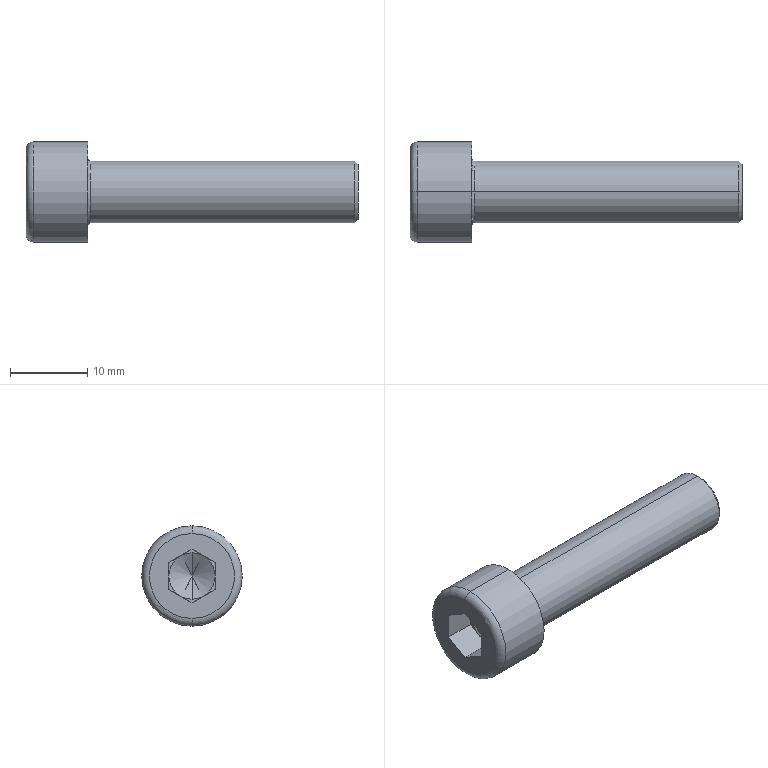Part | SolidWorks | features BaseBody 1 | 1 solid | 27 faces | box 43 x 13 x 13 mm | volume 2671 mm3 | plane 15 | cylinder 4 | torus 4 | cone 4 | commonest cylinder face diameters 8 x2 13 x2
STEP:
#1=CARTESIAN_POINT('',(42.6,0.,4.));
#2=VERTEX_POINT('',#1);
#3=CARTESIAN_POINT('',(42.6,0.,-4.));
#4=VERTEX_POINT('',#3);
#5=CARTESIAN_POINT('',(42.6,0.,0.));
#6=DIRECTION('',(-1.,0.,0.));
#7=DIRECTION('',(0.,0.,1.));
#8=AXIS2_PLACEMENT_3D('',#5,#6,#7);
#9=CIRCLE('',#8,4.);
#10=EDGE_CURVE('',#2,#4,#9,.T.);
#11=ORIENTED_EDGE('',*,*,#10,.T.);
#12=CARTESIAN_POINT('',(8.4,0.,-4.));
#13=VERTEX_POINT('',#12);
#14=CARTESIAN_POINT('',(43.,0.,-4.));
#15=DIRECTION('',(-1.,0.,0.));
#16=VECTOR('',#15,1000.);
#17=LINE('',#14,#16);
#18=EDGE_CURVE('',#4,#13,#17,.T.);
#19=ORIENTED_EDGE('',*,*,#18,.T.);
#20=CARTESIAN_POINT('',(8.4,0.,4.));
#21=VERTEX_POINT('',#20);
#22=CARTESIAN_POINT('',(8.4,0.,0.));
#23=DIRECTION('',(1.,0.,0.));
#24=DIRECTION('',(0.,0.,1.));
#25=AXIS2_PLACEMENT_3D('',#22,#23,#24);
#26=CIRCLE('',#25,4.);
#27=EDGE_CURVE('',#13,#21,#26,.T.);
#28=ORIENTED_EDGE('',*,*,#27,.T.);
#29=CARTESIAN_POINT('',(43.,0.,4.));
#30=DIRECTION('',(-1.,0.,0.));
#31=VECTOR('',#30,1000.);
#32=LINE('',#29,#31);
#33=EDGE_CURVE('',#2,#21,#32,.T.);
#34=ORIENTED_EDGE('',*,*,#33,.F.);
#35=EDGE_LOOP('',(#11,#19,#28,#34));
#36=FACE_OUTER_BOUND('',#35,.T.);
#37=CARTESIAN_POINT('',(43.,0.,0.));
#38=DIRECTION('',(-1.,0.,0.));
#39=DIRECTION('',(0.,0.,1.));
#40=AXIS2_PLACEMENT_3D('',#37,#38,#39);
#41=CYLINDRICAL_SURFACE('',#40,4.);
#42=ADVANCED_FACE('',(#36),#41,.T.);
#43=CARTESIAN_POINT('',(8.4,0.,0.));
#44=DIRECTION('',(1.,0.,0.));
#45=DIRECTION('',(0.,0.,1.));
#46=AXIS2_PLACEMENT_3D('',#43,#44,#45);
#47=CIRCLE('',#46,4.);
#48=EDGE_CURVE('',#21,#13,#47,.T.);
#49=ORIENTED_EDGE('',*,*,#48,.F.);
#50=CARTESIAN_POINT('',(8.,0.,4.4));
#51=VERTEX_POINT('',#50);
#52=CARTESIAN_POINT('',(8.4,0.,4.4));
#53=DIRECTION('',(0.,1.,0.));
#54=DIRECTION('',(0.,0.,1.));
#55=AXIS2_PLACEMENT_3D('',#52,#53,#54);
#56=CIRCLE('',#55,0.4);
#57=EDGE_CURVE('',#21,#51,#56,.T.);
#58=ORIENTED_EDGE('',*,*,#57,.T.);
#59=CARTESIAN_POINT('',(8.,0.,-4.4));
#60=VERTEX_POINT('',#59);
#61=CARTESIAN_POINT('',(8.,0.,-4.4));
#62=CARTESIAN_POINT('',(8.,-0.2798,-4.4));
#63=CARTESIAN_POINT('',(8.,-0.692,-4.361));
#64=CARTESIAN_POINT('',(8.,-1.16,-4.249));
#65=CARTESIAN_POINT('',(8.,-1.391,-4.175));
#66=CARTESIAN_POINT('',(8.,-1.489,-4.141));
#67=CARTESIAN_POINT('',(8.,-1.555,-4.116));
#68=CARTESIAN_POINT('',(8.,-1.585,-4.105));
#69=CARTESIAN_POINT('',(8.,-1.758,-4.036));
#70=CARTESIAN_POINT('',(8.,-1.96,-3.945));
#71=CARTESIAN_POINT('',(8.,-2.154,-3.837));
#72=CARTESIAN_POINT('',(8.,-2.282,-3.763));
#73=CARTESIAN_POINT('',(8.,-2.344,-3.724));
#74=CARTESIAN_POINT('',(8.,-2.661,-3.517));
#75=CARTESIAN_POINT('',(8.,-2.897,-3.326));
#76=CARTESIAN_POINT('',(8.,-3.218,-3.004));
#77=CARTESIAN_POINT('',(8.,-3.37,-2.836));
#78=CARTESIAN_POINT('',(8.,-3.509,-2.656));
#79=CARTESIAN_POINT('',(8.,-3.598,-2.534));
#80=CARTESIAN_POINT('',(8.,-3.642,-2.47));
#81=CARTESIAN_POINT('',(8.,-3.764,-2.284));
#82=CARTESIAN_POINT('',(8.,-3.876,-2.092));
#83=CARTESIAN_POINT('',(8.,-3.989,-1.859));
#84=CARTESIAN_POINT('',(8.,-4.042,-1.74));
#85=CARTESIAN_POINT('',(8.,-4.063,-1.689));
#86=CARTESIAN_POINT('',(8.,-4.077,-1.654));
#87=CARTESIAN_POINT('',(8.,-4.085,-1.636));
#88=CARTESIAN_POINT('',(8.,-4.297,-1.1));
#89=CARTESIAN_POINT('',(8.,-4.4,-0.5588));
#90=CARTESIAN_POINT('',(8.,-4.4,0.2794));
#91=CARTESIAN_POINT('',(8.,-4.361,0.6914));
#92=CARTESIAN_POINT('',(8.,-4.249,1.16));
#93=CARTESIAN_POINT('',(8.,-4.176,1.391));
#94=CARTESIAN_POINT('',(8.,-4.141,1.489));
#95=CARTESIAN_POINT('',(8.,-4.116,1.554));
#96=CARTESIAN_POINT('',(8.,-4.105,1.585));
#97=CARTESIAN_POINT('',(8.,-4.036,1.758));
#98=CARTESIAN_POINT('',(8.,-3.945,1.96));
#99=CARTESIAN_POINT('',(8.,-3.837,2.154));
#100=CARTESIAN_POINT('',(8.,-3.763,2.282));
#101=CARTESIAN_POINT('',(8.,-3.724,2.344));
#102=CARTESIAN_POINT('',(8.,-3.517,2.661));
#103=CARTESIAN_POINT('',(8.,-3.326,2.897));
#104=CARTESIAN_POINT('',(8.,-3.004,3.218));
#105=CARTESIAN_POINT('',(8.,-2.836,3.37));
#106=CARTESIAN_POINT('',(8.,-2.656,3.509));
#107=CARTESIAN_POINT('',(8.,-2.534,3.598));
#108=CARTESIAN_POINT('',(8.,-2.47,3.642));
#109=CARTESIAN_POINT('',(8.,-2.284,3.764));
#110=CARTESIAN_POINT('',(8.,-2.092,3.876));
#111=CARTESIAN_POINT('',(8.,-1.859,3.989));
#112=CARTESIAN_POINT('',(8.,-1.74,4.042));
#113=CARTESIAN_POINT('',(8.,-1.689,4.063));
#114=CARTESIAN_POINT('',(8.,-1.654,4.077));
#115=CARTESIAN_POINT('',(8.,-1.636,4.085));
#116=CARTESIAN_POINT('',(8.,-1.1,4.297));
#117=CARTESIAN_POINT('',(8.,-0.5602,4.4));
#118=CARTESIAN_POINT('',(8.,0.,4.4));
#119=B_SPLINE_CURVE_WITH_KNOTS('',3,(#61,#62,#63,#64,#65,#66,#67,#68,#69,#70,#71,#72,#73,#74,#75,#76,#77,#78,#79,#80,#81,#82,#83,#84,#85,#86,#87,#88,#89,#90,#91,#92,#93,#94,#95,#96,#97,#98,#99,#100,#101,#102,#103,#104,#105,#106,#107,#108,#109,#110,#111,#112,#113,#114,#115,#116,#117,#118),.UNSPECIFIED.,.F.,.F.,(4,1,1,1,2,2,1,2,2,2,1,2,2,1,1,1,2,2,2,1,1,1,2,2,1,2,2,2,1,2,2,1,1,1,2,2,4),(0.,0.0625,0.09375,0.1094,0.1172,0.125,0.1563,0.1719,0.1875,0.25,0.2813,0.2969,0.3125,0.3438,0.3594,0.3672,0.3711,0.375,0.5,0.5625,0.5937,0.6094,0.6172,0.625,0.6562,0.6719,0.6875,0.75,0.7813,0.7969,0.8125,0.8438,0.8594,0.8672,0.8711,0.875,1.),.UNSPECIFIED.);
#120=EDGE_CURVE('',#60,#51,#119,.T.);
#121=ORIENTED_EDGE('',*,*,#120,.F.);
#122=CARTESIAN_POINT('',(8.4,0.,-4.4));
#123=DIRECTION('',(0.,-1.,0.));
#124=DIRECTION('',(0.,0.,-1.));
#125=AXIS2_PLACEMENT_3D('',#122,#123,#124);
#126=CIRCLE('',#125,0.4);
#127=EDGE_CURVE('',#13,#60,#126,.T.);
#128=ORIENTED_EDGE('',*,*,#127,.F.);
#129=EDGE_LOOP('',(#49,#58,#121,#128));
#130=FACE_OUTER_BOUND('',#129,.T.);
#131=CARTESIAN_POINT('',(8.4,0.,0.));
#132=DIRECTION('',(1.,0.,0.));
#133=DIRECTION('',(0.,0.,-1.));
#134=AXIS2_PLACEMENT_3D('',#131,#132,#133);
#135=TOROIDAL_SURFACE('',#134,4.4,0.4);
#136=ADVANCED_FACE('',(#130),#135,.F.);
#137=CARTESIAN_POINT('',(43.,0.,3.6));
#138=VERTEX_POINT('',#137);
#139=CARTESIAN_POINT('',(43.,0.,-3.6));
#140=VERTEX_POINT('',#139);
#141=CARTESIAN_POINT('',(43.,0.,0.));
#142=DIRECTION('',(-1.,0.,0.));
#143=DIRECTION('',(0.,0.,1.));
#144=AXIS2_PLACEMENT_3D('',#141,#142,#143);
#145=CIRCLE('',#144,3.6);
#146=EDGE_CURVE('',#138,#140,#145,.T.);
#147=ORIENTED_EDGE('',*,*,#146,.T.);
#148=CARTESIAN_POINT('',(42.6,0.,-4.));
#149=DIRECTION('',(-0.7071,0.,-0.7071));
#150=VECTOR('',#149,1000.);
#151=LINE('',#148,#150);
#152=EDGE_CURVE('',#140,#4,#151,.T.);
#153=ORIENTED_EDGE('',*,*,#152,.T.);
#154=ORIENTED_EDGE('',*,*,#10,.F.);
#155=CARTESIAN_POINT('',(42.6,0.,4.));
#156=DIRECTION('',(-0.7071,0.,0.7071));
#157=VECTOR('',#156,1000.);
#158=LINE('',#155,#157);
#159=EDGE_CURVE('',#138,#2,#158,.T.);
#160=ORIENTED_EDGE('',*,*,#159,.F.);
#161=EDGE_LOOP('',(#147,#153,#154,#160));
#162=FACE_OUTER_BOUND('',#161,.T.);
#163=CARTESIAN_POINT('',(42.6,0.,0.));
#164=DIRECTION('',(-1.,0.,0.));
#165=DIRECTION('',(0.,0.,1.));
#166=AXIS2_PLACEMENT_3D('',#163,#164,#165);
#167=CONICAL_SURFACE('',#166,4.,0.7854);
#168=ADVANCED_FACE('',(#162),#167,.T.);
#169=CARTESIAN_POINT('',(8.,0.,-6.5));
#170=VERTEX_POINT('',#169);
#171=CARTESIAN_POINT('',(8.,0.,6.5));
#172=VERTEX_POINT('',#171);
#173=CARTESIAN_POINT('',(8.,0.,0.));
#174=DIRECTION('',(1.,0.,0.));
#175=DIRECTION('',(0.,0.,1.));
#176=AXIS2_PLACEMENT_3D('',#173,#174,#175);
#177=CIRCLE('',#176,6.5);
#178=EDGE_CURVE('',#170,#172,#177,.T.);
#179=ORIENTED_EDGE('',*,*,#178,.F.);
#180=CARTESIAN_POINT('',(1.,0.,-6.5));
#181=VERTEX_POINT('',#180);
#182=CARTESIAN_POINT('',(8.,0.,-6.5));
#183=DIRECTION('',(-1.,0.,0.));
#184=VECTOR('',#183,1000.);
#185=LINE('',#182,#184);
#186=EDGE_CURVE('',#170,#181,#185,.T.);
#187=ORIENTED_EDGE('',*,*,#186,.T.);
#188=CARTESIAN_POINT('',(1.,0.,6.5));
#189=VERTEX_POINT('',#188);
#190=CARTESIAN_POINT('',(1.,0.,0.));
#191=DIRECTION('',(1.,0.,0.));
#192=DIRECTION('',(0.,0.,1.));
#193=AXIS2_PLACEMENT_3D('',#190,#191,#192);
#194=CIRCLE('',#193,6.5);
#195=EDGE_CURVE('',#181,#189,#194,.T.);
#196=ORIENTED_EDGE('',*,*,#195,.T.);
#197=CARTESIAN_POINT('',(8.,0.,6.5));
#198=DIRECTION('',(-1.,0.,0.));
#199=VECTOR('',#198,1000.);
#200=LINE('',#197,#199);
#201=EDGE_CURVE('',#172,#189,#200,.T.);
#202=ORIENTED_EDGE('',*,*,#201,.F.);
#203=EDGE_LOOP('',(#179,#187,#196,#202));
#204=FACE_OUTER_BOUND('',#203,.T.);
#205=CARTESIAN_POINT('',(8.,0.,0.));
#206=DIRECTION('',(-1.,0.,0.));
#207=DIRECTION('',(0.,0.,1.));
#208=AXIS2_PLACEMENT_3D('',#205,#206,#207);
#209=CYLINDRICAL_SURFACE('',#208,6.5);
#210=ADVANCED_FACE('',(#204),#209,.T.);
#211=CARTESIAN_POINT('',(0.,0.,-5.5));
#212=VERTEX_POINT('',#211);
#213=CARTESIAN_POINT('',(0.,0.,5.5));
#214=VERTEX_POINT('',#213);
#215=CARTESIAN_POINT('',(0.,0.,0.));
#216=DIRECTION('',(1.,0.,0.));
#217=DIRECTION('',(0.,0.,-1.));
#218=AXIS2_PLACEMENT_3D('',#215,#216,#217);
#219=CIRCLE('',#218,5.5);
#220=EDGE_CURVE('',#212,#214,#219,.T.);
#221=ORIENTED_EDGE('',*,*,#220,.T.);
#222=CARTESIAN_POINT('',(1.,0.,5.5));
#223=DIRECTION('',(0.,1.,0.));
#224=DIRECTION('',(0.,0.,1.));
#225=AXIS2_PLACEMENT_3D('',#222,#223,#224);
#226=CIRCLE('',#225,1.);
#227=EDGE_CURVE('',#214,#189,#226,.T.);
#228=ORIENTED_EDGE('',*,*,#227,.T.);
#229=ORIENTED_EDGE('',*,*,#195,.F.);
#230=CARTESIAN_POINT('',(1.,0.,-5.5));
#231=DIRECTION('',(0.,-1.,0.));
#232=DIRECTION('',(0.,0.,-1.));
#233=AXIS2_PLACEMENT_3D('',#230,#231,#232);
#234=CIRCLE('',#233,1.);
#235=EDGE_CURVE('',#212,#181,#234,.T.);
#236=ORIENTED_EDGE('',*,*,#235,.F.);
#237=EDGE_LOOP('',(#221,#228,#229,#236));
#238=FACE_OUTER_BOUND('',#237,.T.);
#239=CARTESIAN_POINT('',(1.,0.,0.));
#240=DIRECTION('',(1.,0.,0.));
#241=DIRECTION('',(0.,0.,-1.));
#242=AXIS2_PLACEMENT_3D('',#239,#240,#241);
#243=TOROIDAL_SURFACE('',#242,5.5,1.);
#244=ADVANCED_FACE('',(#238),#243,.T.);
#245=CARTESIAN_POINT('',(5.732,0.,0.));
#246=VERTEX_POINT('',#245);
#247=CARTESIAN_POINT('',(4.,0.,3.));
#248=VERTEX_POINT('',#247);
#249=CARTESIAN_POINT('',(4.,0.,3.));
#250=DIRECTION('',(-0.5,0.,0.866));
#251=VECTOR('',#250,1000.);
#252=LINE('',#249,#251);
#253=EDGE_CURVE('',#246,#248,#252,.T.);
#254=ORIENTED_EDGE('',*,*,#253,.F.);
#255=CARTESIAN_POINT('',(4.,0.,-3.));
#256=VERTEX_POINT('',#255);
#257=CARTESIAN_POINT('',(4.,0.,-3.));
#258=DIRECTION('',(-0.5,0.,-0.866));
#259=VECTOR('',#258,1000.);
#260=LINE('',#257,#259);
#261=EDGE_CURVE('',#246,#256,#260,.T.);
#262=ORIENTED_EDGE('',*,*,#261,.T.);
#263=CARTESIAN_POINT('',(4.,-1.5,-2.598));
#264=VERTEX_POINT('',#263);
#265=CARTESIAN_POINT('',(4.,0.,0.));
#266=DIRECTION('',(1.,0.,0.));
#267=DIRECTION('',(0.,0.,1.));
#268=AXIS2_PLACEMENT_3D('',#265,#266,#267);
#269=CIRCLE('',#268,3.);
#270=EDGE_CURVE('',#264,#256,#269,.T.);
#271=ORIENTED_EDGE('',*,*,#270,.F.);
#272=CARTESIAN_POINT('',(4.,-3.,0.));
#273=VERTEX_POINT('',#272);
#274=CARTESIAN_POINT('',(4.,0.,0.));
#275=DIRECTION('',(-1.,0.,0.));
#276=DIRECTION('',(0.,0.,1.));
#277=AXIS2_PLACEMENT_3D('',#274,#275,#276);
#278=CIRCLE('',#277,3.);
#279=EDGE_CURVE('',#264,#273,#278,.T.);
#280=ORIENTED_EDGE('',*,*,#279,.T.);
#281=CARTESIAN_POINT('',(4.,-1.5,2.598));
#282=VERTEX_POINT('',#281);
#283=CARTESIAN_POINT('',(4.,0.,0.));
#284=DIRECTION('',(1.,0.,0.));
#285=DIRECTION('',(0.,0.,1.));
#286=AXIS2_PLACEMENT_3D('',#283,#284,#285);
#287=CIRCLE('',#286,3.);
#288=EDGE_CURVE('',#282,#273,#287,.T.);
#289=ORIENTED_EDGE('',*,*,#288,.F.);
#290=CARTESIAN_POINT('',(4.,0.,0.));
#291=DIRECTION('',(1.,0.,0.));
#292=DIRECTION('',(0.,0.,1.));
#293=AXIS2_PLACEMENT_3D('',#290,#291,#292);
#294=CIRCLE('',#293,3.);
#295=EDGE_CURVE('',#248,#282,#294,.T.);
#296=ORIENTED_EDGE('',*,*,#295,.F.);
#297=EDGE_LOOP('',(#254,#262,#271,#280,#289,#296));
#298=FACE_OUTER_BOUND('',#297,.T.);
#299=CARTESIAN_POINT('',(4.,0.,0.));
#300=DIRECTION('',(-1.,0.,0.));
#301=DIRECTION('',(0.,0.,1.));
#302=AXIS2_PLACEMENT_3D('',#299,#300,#301);
#303=CONICAL_SURFACE('',#302,3.,1.047);
#304=ADVANCED_FACE('',(#298),#303,.F.);
#305=ORIENTED_EDGE('',*,*,#18,.F.);
#306=CARTESIAN_POINT('',(42.6,0.,0.));
#307=DIRECTION('',(-1.,0.,0.));
#308=DIRECTION('',(0.,0.,1.));
#309=AXIS2_PLACEMENT_3D('',#306,#307,#308);
#310=CIRCLE('',#309,4.);
#311=EDGE_CURVE('',#4,#2,#310,.T.);
#312=ORIENTED_EDGE('',*,*,#311,.T.);
#313=ORIENTED_EDGE('',*,*,#33,.T.);
#314=ORIENTED_EDGE('',*,*,#48,.T.);
#315=EDGE_LOOP('',(#305,#312,#313,#314));
#316=FACE_OUTER_BOUND('',#315,.T.);
#317=CARTESIAN_POINT('',(43.,0.,0.));
#318=DIRECTION('',(-1.,0.,0.));
#319=DIRECTION('',(0.,0.,1.));
#320=AXIS2_PLACEMENT_3D('',#317,#318,#319);
#321=CYLINDRICAL_SURFACE('',#320,4.);
#322=ADVANCED_FACE('',(#316),#321,.T.);
#323=ORIENTED_EDGE('',*,*,#57,.F.);
#324=ORIENTED_EDGE('',*,*,#27,.F.);
#325=ORIENTED_EDGE('',*,*,#127,.T.);
#326=CARTESIAN_POINT('',(8.,0.,4.4));
#327=CARTESIAN_POINT('',(8.,0.2798,4.4));
#328=CARTESIAN_POINT('',(8.,0.692,4.361));
#329=CARTESIAN_POINT('',(8.,1.16,4.249));
#330=CARTESIAN_POINT('',(8.,1.391,4.175));
#331=CARTESIAN_POINT('',(8.,1.489,4.141));
#332=CARTESIAN_POINT('',(8.,1.555,4.116));
#333=CARTESIAN_POINT('',(8.,1.585,4.105));
#334=CARTESIAN_POINT('',(8.,1.758,4.036));
#335=CARTESIAN_POINT('',(8.,1.96,3.945));
#336=CARTESIAN_POINT('',(8.,2.154,3.837));
#337=CARTESIAN_POINT('',(8.,2.282,3.763));
#338=CARTESIAN_POINT('',(8.,2.344,3.724));
#339=CARTESIAN_POINT('',(8.,2.661,3.517));
#340=CARTESIAN_POINT('',(8.,2.897,3.326));
#341=CARTESIAN_POINT('',(8.,3.218,3.004));
#342=CARTESIAN_POINT('',(8.,3.37,2.836));
#343=CARTESIAN_POINT('',(8.,3.509,2.656));
#344=CARTESIAN_POINT('',(8.,3.598,2.534));
#345=CARTESIAN_POINT('',(8.,3.642,2.47));
#346=CARTESIAN_POINT('',(8.,3.764,2.284));
#347=CARTESIAN_POINT('',(8.,3.876,2.092));
#348=CARTESIAN_POINT('',(8.,3.989,1.859));
#349=CARTESIAN_POINT('',(8.,4.042,1.74));
#350=CARTESIAN_POINT('',(8.,4.063,1.689));
#351=CARTESIAN_POINT('',(8.,4.077,1.654));
#352=CARTESIAN_POINT('',(8.,4.085,1.636));
#353=CARTESIAN_POINT('',(8.,4.297,1.1));
#354=CARTESIAN_POINT('',(8.,4.4,0.5588));
#355=CARTESIAN_POINT('',(8.,4.4,-0.2794));
#356=CARTESIAN_POINT('',(8.,4.361,-0.6914));
#357=CARTESIAN_POINT('',(8.,4.249,-1.16));
#358=CARTESIAN_POINT('',(8.,4.176,-1.391));
#359=CARTESIAN_POINT('',(8.,4.141,-1.489));
#360=CARTESIAN_POINT('',(8.,4.116,-1.554));
#361=CARTESIAN_POINT('',(8.,4.105,-1.585));
#362=CARTESIAN_POINT('',(8.,4.036,-1.758));
#363=CARTESIAN_POINT('',(8.,3.945,-1.96));
#364=CARTESIAN_POINT('',(8.,3.837,-2.154));
#365=CARTESIAN_POINT('',(8.,3.763,-2.282));
#366=CARTESIAN_POINT('',(8.,3.724,-2.344));
#367=CARTESIAN_POINT('',(8.,3.517,-2.661));
#368=CARTESIAN_POINT('',(8.,3.326,-2.897));
#369=CARTESIAN_POINT('',(8.,3.004,-3.218));
#370=CARTESIAN_POINT('',(8.,2.836,-3.37));
#371=CARTESIAN_POINT('',(8.,2.656,-3.509));
#372=CARTESIAN_POINT('',(8.,2.534,-3.598));
#373=CARTESIAN_POINT('',(8.,2.47,-3.642));
#374=CARTESIAN_POINT('',(8.,2.284,-3.764));
#375=CARTESIAN_POINT('',(8.,2.092,-3.876));
#376=CARTESIAN_POINT('',(8.,1.859,-3.989));
#377=CARTESIAN_POINT('',(8.,1.74,-4.042));
#378=CARTESIAN_POINT('',(8.,1.689,-4.063));
#379=CARTESIAN_POINT('',(8.,1.654,-4.077));
#380=CARTESIAN_POINT('',(8.,1.636,-4.085));
#381=CARTESIAN_POINT('',(8.,1.1,-4.297));
#382=CARTESIAN_POINT('',(8.,0.5602,-4.4));
#383=CARTESIAN_POINT('',(8.,0.,-4.4));
#384=B_SPLINE_CURVE_WITH_KNOTS('',3,(#326,#327,#328,#329,#330,#331,#332,#333,#334,#335,#336,#337,#338,#339,#340,#341,#342,#343,#344,#345,#346,#347,#348,#349,#350,#351,#352,#353,#354,#355,#356,#357,#358,#359,#360,#361,#362,#363,#364,#365,#366,#367,#368,#369,#370,#371,#372,#373,#374,#375,#376,#377,#378,#379,#380,#381,#382,#383),.UNSPECIFIED.,.F.,.F.,(4,1,1,1,2,2,1,2,2,2,1,2,2,1,1,1,2,2,2,1,1,1,2,2,1,2,2,2,1,2,2,1,1,1,2,2,4),(0.,0.0625,0.09375,0.1094,0.1172,0.125,0.1563,0.1719,0.1875,0.25,0.2813,0.2969,0.3125,0.3438,0.3594,0.3672,0.3711,0.375,0.5,0.5625,0.5937,0.6094,0.6172,0.625,0.6562,0.6719,0.6875,0.75,0.7812,0.7969,0.8125,0.8437,0.8594,0.8672,0.8711,0.875,1.),.UNSPECIFIED.);
#385=EDGE_CURVE('',#51,#60,#384,.T.);
#386=ORIENTED_EDGE('',*,*,#385,.F.);
#387=EDGE_LOOP('',(#323,#324,#325,#386));
#388=FACE_OUTER_BOUND('',#387,.T.);
#389=CARTESIAN_POINT('',(8.4,0.,0.));
#390=DIRECTION('',(1.,0.,0.));
#391=DIRECTION('',(0.,0.,-1.));
#392=AXIS2_PLACEMENT_3D('',#389,#390,#391);
#393=TOROIDAL_SURFACE('',#392,4.4,0.4);
#394=ADVANCED_FACE('',(#388),#393,.F.);
#395=ORIENTED_EDGE('',*,*,#152,.F.);
#396=CARTESIAN_POINT('',(43.,0.,0.));
#397=DIRECTION('',(-1.,0.,0.));
#398=DIRECTION('',(0.,0.,1.));
#399=AXIS2_PLACEMENT_3D('',#396,#397,#398);
#400=CIRCLE('',#399,3.6);
#401=EDGE_CURVE('',#140,#138,#400,.T.);
#402=ORIENTED_EDGE('',*,*,#401,.T.);
#403=ORIENTED_EDGE('',*,*,#159,.T.);
#404=ORIENTED_EDGE('',*,*,#311,.F.);
#405=EDGE_LOOP('',(#395,#402,#403,#404));
#406=FACE_OUTER_BOUND('',#405,.T.);
#407=CARTESIAN_POINT('',(42.6,0.,0.));
#408=DIRECTION('',(-1.,0.,0.));
#409=DIRECTION('',(0.,0.,1.));
#410=AXIS2_PLACEMENT_3D('',#407,#408,#409);
#411=CONICAL_SURFACE('',#410,4.,0.7854);
#412=ADVANCED_FACE('',(#406),#411,.T.);
#413=ORIENTED_EDGE('',*,*,#120,.T.);
#414=ORIENTED_EDGE('',*,*,#385,.T.);
#415=EDGE_LOOP('',(#413,#414));
#416=FACE_BOUND('',#415,.T.);
#417=CARTESIAN_POINT('',(8.,0.,0.));
#418=DIRECTION('',(1.,0.,0.));
#419=DIRECTION('',(0.,0.,1.));
#420=AXIS2_PLACEMENT_3D('',#417,#418,#419);
#421=CIRCLE('',#420,6.5);
#422=EDGE_CURVE('',#172,#170,#421,.T.);
#423=ORIENTED_EDGE('',*,*,#422,.T.);
#424=ORIENTED_EDGE('',*,*,#178,.T.);
#425=EDGE_LOOP('',(#423,#424));
#426=FACE_OUTER_BOUND('',#425,.T.);
#427=CARTESIAN_POINT('',(8.,0.,0.));
#428=DIRECTION('',(1.,0.,0.));
#429=DIRECTION('',(0.,0.,-1.));
#430=AXIS2_PLACEMENT_3D('',#427,#428,#429);
#431=PLANE('',#430);
#432=ADVANCED_FACE('',(#416,#426),#431,.T.);
#433=ORIENTED_EDGE('',*,*,#146,.F.);
#434=ORIENTED_EDGE('',*,*,#401,.F.);
#435=EDGE_LOOP('',(#433,#434));
#436=FACE_OUTER_BOUND('',#435,.T.);
#437=CARTESIAN_POINT('',(43.,0.,0.));
#438=DIRECTION('',(1.,0.,0.));
#439=DIRECTION('',(0.,0.,-1.));
#440=AXIS2_PLACEMENT_3D('',#437,#438,#439);
#441=PLANE('',#440);
#442=ADVANCED_FACE('',(#436),#441,.T.);
#443=ORIENTED_EDGE('',*,*,#186,.F.);
#444=ORIENTED_EDGE('',*,*,#422,.F.);
#445=ORIENTED_EDGE('',*,*,#201,.T.);
#446=CARTESIAN_POINT('',(1.,0.,0.));
#447=DIRECTION('',(1.,0.,0.));
#448=DIRECTION('',(0.,0.,1.));
#449=AXIS2_PLACEMENT_3D('',#446,#447,#448);
#450=CIRCLE('',#449,6.5);
#451=EDGE_CURVE('',#189,#181,#450,.T.);
#452=ORIENTED_EDGE('',*,*,#451,.T.);
#453=EDGE_LOOP('',(#443,#444,#445,#452));
#454=FACE_OUTER_BOUND('',#453,.T.);
#455=CARTESIAN_POINT('',(8.,0.,0.));
#456=DIRECTION('',(-1.,0.,0.));
#457=DIRECTION('',(0.,0.,1.));
#458=AXIS2_PLACEMENT_3D('',#455,#456,#457);
#459=CYLINDRICAL_SURFACE('',#458,6.5);
#460=ADVANCED_FACE('',(#454),#459,.T.);
#461=ORIENTED_EDGE('',*,*,#227,.F.);
#462=CARTESIAN_POINT('',(0.,0.,0.));
#463=DIRECTION('',(1.,0.,0.));
#464=DIRECTION('',(0.,0.,-1.));
#465=AXIS2_PLACEMENT_3D('',#462,#463,#464);
#466=CIRCLE('',#465,5.5);
#467=EDGE_CURVE('',#214,#212,#466,.T.);
#468=ORIENTED_EDGE('',*,*,#467,.T.);
#469=ORIENTED_EDGE('',*,*,#235,.T.);
#470=ORIENTED_EDGE('',*,*,#451,.F.);
#471=EDGE_LOOP('',(#461,#468,#469,#470));
#472=FACE_OUTER_BOUND('',#471,.T.);
#473=CARTESIAN_POINT('',(1.,0.,0.));
#474=DIRECTION('',(1.,0.,0.));
#475=DIRECTION('',(0.,0.,-1.));
#476=AXIS2_PLACEMENT_3D('',#473,#474,#475);
#477=TOROIDAL_SURFACE('',#476,5.5,1.);
#478=ADVANCED_FACE('',(#472),#477,.T.);
#479=ORIENTED_EDGE('',*,*,#220,.F.);
#480=ORIENTED_EDGE('',*,*,#467,.F.);
#481=EDGE_LOOP('',(#479,#480));
#482=FACE_OUTER_BOUND('',#481,.T.);
#483=CARTESIAN_POINT('',(0.,3.,1.732));
#484=VERTEX_POINT('',#483);
#485=CARTESIAN_POINT('',(0.,3.,-1.732));
#486=VERTEX_POINT('',#485);
#487=CARTESIAN_POINT('',(0.,3.,0.));
#488=DIRECTION('',(0.,0.,-1.));
#489=VECTOR('',#488,1000.);
#490=LINE('',#487,#489);
#491=EDGE_CURVE('',#484,#486,#490,.T.);
#492=ORIENTED_EDGE('',*,*,#491,.F.);
#493=CARTESIAN_POINT('',(0.,0.,3.464));
#494=VERTEX_POINT('',#493);
#495=CARTESIAN_POINT('',(0.,0.,3.464));
#496=DIRECTION('',(0.,0.866,-0.5));
#497=VECTOR('',#496,1000.);
#498=LINE('',#495,#497);
#499=EDGE_CURVE('',#494,#484,#498,.T.);
#500=ORIENTED_EDGE('',*,*,#499,.F.);
#501=CARTESIAN_POINT('',(0.,-3.,1.732));
#502=VERTEX_POINT('',#501);
#503=CARTESIAN_POINT('',(0.,-3.,1.732));
#504=DIRECTION('',(0.,0.866,0.5));
#505=VECTOR('',#504,1000.);
#506=LINE('',#503,#505);
#507=EDGE_CURVE('',#502,#494,#506,.T.);
#508=ORIENTED_EDGE('',*,*,#507,.F.);
#509=CARTESIAN_POINT('',(0.,-3.,-1.732));
#510=VERTEX_POINT('',#509);
#511=CARTESIAN_POINT('',(0.,-3.,0.));
#512=DIRECTION('',(0.,0.,1.));
#513=VECTOR('',#512,1000.);
#514=LINE('',#511,#513);
#515=EDGE_CURVE('',#510,#502,#514,.T.);
#516=ORIENTED_EDGE('',*,*,#515,.F.);
#517=CARTESIAN_POINT('',(0.,0.,-3.464));
#518=VERTEX_POINT('',#517);
#519=CARTESIAN_POINT('',(0.,0.,-3.464));
#520=DIRECTION('',(0.,-0.866,0.5));
#521=VECTOR('',#520,1000.);
#522=LINE('',#519,#521);
#523=EDGE_CURVE('',#518,#510,#522,.T.);
#524=ORIENTED_EDGE('',*,*,#523,.F.);
#525=CARTESIAN_POINT('',(0.,3.,-1.732));
#526=DIRECTION('',(0.,-0.866,-0.5));
#527=VECTOR('',#526,1000.);
#528=LINE('',#525,#527);
#529=EDGE_CURVE('',#486,#518,#528,.T.);
#530=ORIENTED_EDGE('',*,*,#529,.F.);
#531=EDGE_LOOP('',(#492,#500,#508,#516,#524,#530));
#532=FACE_BOUND('',#531,.T.);
#533=CARTESIAN_POINT('',(0.,0.,0.));
#534=DIRECTION('',(1.,0.,0.));
#535=DIRECTION('',(0.,0.,-1.));
#536=AXIS2_PLACEMENT_3D('',#533,#534,#535);
#537=PLANE('',#536);
#538=ADVANCED_FACE('',(#482,#532),#537,.F.);
#539=CARTESIAN_POINT('',(4.,0.,-3.464));
#540=VERTEX_POINT('',#539);
#541=CARTESIAN_POINT('',(4.,0.,-3.464));
#542=DIRECTION('',(1.,0.,0.));
#543=VECTOR('',#542,1000.);
#544=LINE('',#541,#543);
#545=EDGE_CURVE('',#518,#540,#544,.T.);
#546=ORIENTED_EDGE('',*,*,#545,.T.);
#547=CARTESIAN_POINT('',(4.,1.5,-2.598));
#548=VERTEX_POINT('',#547);
#549=CARTESIAN_POINT('',(4.,0.,-3.464));
#550=DIRECTION('',(0.,0.866,0.5));
#551=VECTOR('',#550,1000.);
#552=LINE('',#549,#551);
#553=EDGE_CURVE('',#540,#548,#552,.T.);
#554=ORIENTED_EDGE('',*,*,#553,.T.);
#555=CARTESIAN_POINT('',(4.,3.,-1.732));
#556=VERTEX_POINT('',#555);
#557=CARTESIAN_POINT('',(4.,1.5,-2.598));
#558=DIRECTION('',(0.,0.866,0.5));
#559=VECTOR('',#558,1000.);
#560=LINE('',#557,#559);
#561=EDGE_CURVE('',#548,#556,#560,.T.);
#562=ORIENTED_EDGE('',*,*,#561,.T.);
#563=CARTESIAN_POINT('',(4.,3.,-1.732));
#564=DIRECTION('',(-1.,0.,0.));
#565=VECTOR('',#564,1000.);
#566=LINE('',#563,#565);
#567=EDGE_CURVE('',#556,#486,#566,.T.);
#568=ORIENTED_EDGE('',*,*,#567,.T.);
#569=ORIENTED_EDGE('',*,*,#529,.T.);
#570=EDGE_LOOP('',(#546,#554,#562,#568,#569));
#571=FACE_OUTER_BOUND('',#570,.T.);
#572=CARTESIAN_POINT('',(4.,0.,-3.464));
#573=DIRECTION('',(0.,-0.5,0.866));
#574=DIRECTION('',(0.,-0.866,-0.5));
#575=AXIS2_PLACEMENT_3D('',#572,#573,#574);
#576=PLANE('',#575);
#577=ADVANCED_FACE('',(#571),#576,.T.);
#578=ORIENTED_EDGE('',*,*,#567,.F.);
#579=CARTESIAN_POINT('',(4.,3.,0.));
#580=VERTEX_POINT('',#579);
#581=CARTESIAN_POINT('',(4.,3.,-3.464));
#582=DIRECTION('',(0.,0.,1.));
#583=VECTOR('',#582,1000.);
#584=LINE('',#581,#583);
#585=EDGE_CURVE('',#556,#580,#584,.T.);
#586=ORIENTED_EDGE('',*,*,#585,.T.);
#587=CARTESIAN_POINT('',(4.,3.,1.732));
#588=VERTEX_POINT('',#587);
#589=CARTESIAN_POINT('',(4.,3.,-3.464));
#590=DIRECTION('',(0.,0.,1.));
#591=VECTOR('',#590,1000.);
#592=LINE('',#589,#591);
#593=EDGE_CURVE('',#580,#588,#592,.T.);
#594=ORIENTED_EDGE('',*,*,#593,.T.);
#595=CARTESIAN_POINT('',(4.,3.,1.732));
#596=DIRECTION('',(-1.,0.,0.));
#597=VECTOR('',#596,1000.);
#598=LINE('',#595,#597);
#599=EDGE_CURVE('',#588,#484,#598,.T.);
#600=ORIENTED_EDGE('',*,*,#599,.T.);
#601=ORIENTED_EDGE('',*,*,#491,.T.);
#602=EDGE_LOOP('',(#578,#586,#594,#600,#601));
#603=FACE_OUTER_BOUND('',#602,.T.);
#604=CARTESIAN_POINT('',(4.,3.,-1.732));
#605=DIRECTION('',(0.,-1.,0.));
#606=DIRECTION('',(0.,0.,-1.));
#607=AXIS2_PLACEMENT_3D('',#604,#605,#606);
#608=PLANE('',#607);
#609=ADVANCED_FACE('',(#603),#608,.T.);
#610=ORIENTED_EDGE('',*,*,#599,.F.);
#611=CARTESIAN_POINT('',(4.,1.5,2.598));
#612=VERTEX_POINT('',#611);
#613=CARTESIAN_POINT('',(4.,3.,1.732));
#614=DIRECTION('',(0.,-0.866,0.5));
#615=VECTOR('',#614,1000.);
#616=LINE('',#613,#615);
#617=EDGE_CURVE('',#588,#612,#616,.T.);
#618=ORIENTED_EDGE('',*,*,#617,.T.);
#619=CARTESIAN_POINT('',(4.,0.,3.464));
#620=VERTEX_POINT('',#619);
#621=CARTESIAN_POINT('',(4.,3.,1.732));
#622=DIRECTION('',(0.,-0.866,0.5));
#623=VECTOR('',#622,1000.);
#624=LINE('',#621,#623);
#625=EDGE_CURVE('',#612,#620,#624,.T.);
#626=ORIENTED_EDGE('',*,*,#625,.T.);
#627=CARTESIAN_POINT('',(4.,0.,3.464));
#628=DIRECTION('',(-1.,0.,0.));
#629=VECTOR('',#628,1000.);
#630=LINE('',#627,#629);
#631=EDGE_CURVE('',#620,#494,#630,.T.);
#632=ORIENTED_EDGE('',*,*,#631,.T.);
#633=ORIENTED_EDGE('',*,*,#499,.T.);
#634=EDGE_LOOP('',(#610,#618,#626,#632,#633));
#635=FACE_OUTER_BOUND('',#634,.T.);
#636=CARTESIAN_POINT('',(4.,3.,1.732));
#637=DIRECTION('',(0.,-0.5,-0.866));
#638=DIRECTION('',(0.,0.866,-0.5));
#639=AXIS2_PLACEMENT_3D('',#636,#637,#638);
#640=PLANE('',#639);
#641=ADVANCED_FACE('',(#635),#640,.T.);
#642=ORIENTED_EDGE('',*,*,#631,.F.);
#643=CARTESIAN_POINT('',(4.,0.,3.464));
#644=DIRECTION('',(0.,-0.866,-0.5));
#645=VECTOR('',#644,1000.);
#646=LINE('',#643,#645);
#647=EDGE_CURVE('',#620,#282,#646,.T.);
#648=ORIENTED_EDGE('',*,*,#647,.T.);
#649=CARTESIAN_POINT('',(4.,-3.,1.732));
#650=VERTEX_POINT('',#649);
#651=CARTESIAN_POINT('',(4.,-1.5,2.598));
#652=DIRECTION('',(0.,-0.866,-0.5));
#653=VECTOR('',#652,1000.);
#654=LINE('',#651,#653);
#655=EDGE_CURVE('',#282,#650,#654,.T.);
#656=ORIENTED_EDGE('',*,*,#655,.T.);
#657=CARTESIAN_POINT('',(4.,-3.,1.732));
#658=DIRECTION('',(-1.,0.,0.));
#659=VECTOR('',#658,1000.);
#660=LINE('',#657,#659);
#661=EDGE_CURVE('',#650,#502,#660,.T.);
#662=ORIENTED_EDGE('',*,*,#661,.T.);
#663=ORIENTED_EDGE('',*,*,#507,.T.);
#664=EDGE_LOOP('',(#642,#648,#656,#662,#663));
#665=FACE_OUTER_BOUND('',#664,.T.);
#666=CARTESIAN_POINT('',(4.,0.,3.464));
#667=DIRECTION('',(0.,0.5,-0.866));
#668=DIRECTION('',(0.,0.866,0.5));
#669=AXIS2_PLACEMENT_3D('',#666,#667,#668);
#670=PLANE('',#669);
#671=ADVANCED_FACE('',(#665),#670,.T.);
#672=ORIENTED_EDGE('',*,*,#661,.F.);
#673=CARTESIAN_POINT('',(4.,-3.,-3.464));
#674=DIRECTION('',(0.,0.,-1.));
#675=VECTOR('',#674,1000.);
#676=LINE('',#673,#675);
#677=EDGE_CURVE('',#650,#273,#676,.T.);
#678=ORIENTED_EDGE('',*,*,#677,.T.);
#679=CARTESIAN_POINT('',(4.,-3.,-1.732));
#680=VERTEX_POINT('',#679);
#681=CARTESIAN_POINT('',(4.,-3.,1.732));
#682=DIRECTION('',(0.,0.,-1.));
#683=VECTOR('',#682,1000.);
#684=LINE('',#681,#683);
#685=EDGE_CURVE('',#273,#680,#684,.T.);
#686=ORIENTED_EDGE('',*,*,#685,.T.);
#687=CARTESIAN_POINT('',(4.,-3.,-1.732));
#688=DIRECTION('',(-1.,0.,0.));
#689=VECTOR('',#688,1000.);
#690=LINE('',#687,#689);
#691=EDGE_CURVE('',#680,#510,#690,.T.);
#692=ORIENTED_EDGE('',*,*,#691,.T.);
#693=ORIENTED_EDGE('',*,*,#515,.T.);
#694=EDGE_LOOP('',(#672,#678,#686,#692,#693));
#695=FACE_OUTER_BOUND('',#694,.T.);
#696=CARTESIAN_POINT('',(4.,-3.,1.732));
#697=DIRECTION('',(0.,1.,0.));
#698=DIRECTION('',(0.,0.,1.));
#699=AXIS2_PLACEMENT_3D('',#696,#697,#698);
#700=PLANE('',#699);
#701=ADVANCED_FACE('',(#695),#700,.T.);
#702=ORIENTED_EDGE('',*,*,#691,.F.);
#703=CARTESIAN_POINT('',(4.,-3.,-1.732));
#704=DIRECTION('',(0.,0.866,-0.5));
#705=VECTOR('',#704,1000.);
#706=LINE('',#703,#705);
#707=EDGE_CURVE('',#680,#264,#706,.T.);
#708=ORIENTED_EDGE('',*,*,#707,.T.);
#709=CARTESIAN_POINT('',(4.,-3.,-1.732));
#710=DIRECTION('',(0.,0.866,-0.5));
#711=VECTOR('',#710,1000.);
#712=LINE('',#709,#711);
#713=EDGE_CURVE('',#264,#540,#712,.T.);
#714=ORIENTED_EDGE('',*,*,#713,.T.);
#715=ORIENTED_EDGE('',*,*,#545,.F.);
#716=ORIENTED_EDGE('',*,*,#523,.T.);
#717=EDGE_LOOP('',(#702,#708,#714,#715,#716));
#718=FACE_OUTER_BOUND('',#717,.T.);
#719=CARTESIAN_POINT('',(4.,-3.,-1.732));
#720=DIRECTION('',(0.,0.5,0.866));
#721=DIRECTION('',(0.,-0.866,0.5));
#722=AXIS2_PLACEMENT_3D('',#719,#720,#721);
#723=PLANE('',#722);
#724=ADVANCED_FACE('',(#718),#723,.T.);
#725=ORIENTED_EDGE('',*,*,#270,.T.);
#726=CARTESIAN_POINT('',(4.,0.,0.));
#727=DIRECTION('',(1.,0.,0.));
#728=DIRECTION('',(0.,0.,1.));
#729=AXIS2_PLACEMENT_3D('',#726,#727,#728);
#730=CIRCLE('',#729,3.);
#731=EDGE_CURVE('',#256,#548,#730,.T.);
#732=ORIENTED_EDGE('',*,*,#731,.T.);
#733=ORIENTED_EDGE('',*,*,#553,.F.);
#734=ORIENTED_EDGE('',*,*,#713,.F.);
#735=EDGE_LOOP('',(#725,#732,#733,#734));
#736=FACE_OUTER_BOUND('',#735,.T.);
#737=CARTESIAN_POINT('',(4.,0.,-3.464));
#738=DIRECTION('',(1.,0.,0.));
#739=DIRECTION('',(0.,0.,-1.));
#740=AXIS2_PLACEMENT_3D('',#737,#738,#739);
#741=PLANE('',#740);
#742=ADVANCED_FACE('',(#736),#741,.F.);
#743=ORIENTED_EDGE('',*,*,#625,.F.);
#744=CARTESIAN_POINT('',(4.,0.,0.));
#745=DIRECTION('',(1.,0.,0.));
#746=DIRECTION('',(0.,0.,1.));
#747=AXIS2_PLACEMENT_3D('',#744,#745,#746);
#748=CIRCLE('',#747,3.);
#749=EDGE_CURVE('',#612,#248,#748,.T.);
#750=ORIENTED_EDGE('',*,*,#749,.T.);
#751=ORIENTED_EDGE('',*,*,#295,.T.);
#752=ORIENTED_EDGE('',*,*,#647,.F.);
#753=EDGE_LOOP('',(#743,#750,#751,#752));
#754=FACE_OUTER_BOUND('',#753,.T.);
#755=CARTESIAN_POINT('',(4.,0.,-3.464));
#756=DIRECTION('',(1.,0.,0.));
#757=DIRECTION('',(0.,0.,-1.));
#758=AXIS2_PLACEMENT_3D('',#755,#756,#757);
#759=PLANE('',#758);
#760=ADVANCED_FACE('',(#754),#759,.F.);
#761=ORIENTED_EDGE('',*,*,#707,.F.);
#762=ORIENTED_EDGE('',*,*,#685,.F.);
#763=ORIENTED_EDGE('',*,*,#279,.F.);
#764=EDGE_LOOP('',(#761,#762,#763));
#765=FACE_OUTER_BOUND('',#764,.T.);
#766=CARTESIAN_POINT('',(4.,0.,-3.464));
#767=DIRECTION('',(1.,0.,0.));
#768=DIRECTION('',(0.,0.,-1.));
#769=AXIS2_PLACEMENT_3D('',#766,#767,#768);
#770=PLANE('',#769);
#771=ADVANCED_FACE('',(#765),#770,.F.);
#772=ORIENTED_EDGE('',*,*,#261,.F.);
#773=ORIENTED_EDGE('',*,*,#253,.T.);
#774=ORIENTED_EDGE('',*,*,#749,.F.);
#775=CARTESIAN_POINT('',(4.,0.,0.));
#776=DIRECTION('',(1.,0.,0.));
#777=DIRECTION('',(0.,0.,1.));
#778=AXIS2_PLACEMENT_3D('',#775,#776,#777);
#779=CIRCLE('',#778,3.);
#780=EDGE_CURVE('',#580,#612,#779,.T.);
#781=ORIENTED_EDGE('',*,*,#780,.F.);
#782=CARTESIAN_POINT('',(4.,0.,0.));
#783=DIRECTION('',(1.,0.,0.));
#784=DIRECTION('',(0.,0.,1.));
#785=AXIS2_PLACEMENT_3D('',#782,#783,#784);
#786=CIRCLE('',#785,3.);
#787=EDGE_CURVE('',#548,#580,#786,.T.);
#788=ORIENTED_EDGE('',*,*,#787,.F.);
#789=ORIENTED_EDGE('',*,*,#731,.F.);
#790=EDGE_LOOP('',(#772,#773,#774,#781,#788,#789));
#791=FACE_OUTER_BOUND('',#790,.T.);
#792=CARTESIAN_POINT('',(4.,0.,0.));
#793=DIRECTION('',(-1.,0.,0.));
#794=DIRECTION('',(0.,0.,1.));
#795=AXIS2_PLACEMENT_3D('',#792,#793,#794);
#796=CONICAL_SURFACE('',#795,3.,1.047);
#797=ADVANCED_FACE('',(#791),#796,.F.);
#798=ORIENTED_EDGE('',*,*,#677,.F.);
#799=ORIENTED_EDGE('',*,*,#655,.F.);
#800=ORIENTED_EDGE('',*,*,#288,.T.);
#801=EDGE_LOOP('',(#798,#799,#800));
#802=FACE_OUTER_BOUND('',#801,.T.);
#803=CARTESIAN_POINT('',(4.,0.,-3.464));
#804=DIRECTION('',(1.,0.,0.));
#805=DIRECTION('',(0.,0.,-1.));
#806=AXIS2_PLACEMENT_3D('',#803,#804,#805);
#807=PLANE('',#806);
#808=ADVANCED_FACE('',(#802),#807,.F.);
#809=ORIENTED_EDGE('',*,*,#617,.F.);
#810=ORIENTED_EDGE('',*,*,#593,.F.);
#811=ORIENTED_EDGE('',*,*,#780,.T.);
#812=EDGE_LOOP('',(#809,#810,#811));
#813=FACE_OUTER_BOUND('',#812,.T.);
#814=CARTESIAN_POINT('',(4.,0.,-3.464));
#815=DIRECTION('',(1.,0.,0.));
#816=DIRECTION('',(0.,0.,-1.));
#817=AXIS2_PLACEMENT_3D('',#814,#815,#816);
#818=PLANE('',#817);
#819=ADVANCED_FACE('',(#813),#818,.F.);
#820=ORIENTED_EDGE('',*,*,#585,.F.);
#821=ORIENTED_EDGE('',*,*,#561,.F.);
#822=ORIENTED_EDGE('',*,*,#787,.T.);
#823=EDGE_LOOP('',(#820,#821,#822));
#824=FACE_OUTER_BOUND('',#823,.T.);
#825=CARTESIAN_POINT('',(4.,0.,-3.464));
#826=DIRECTION('',(1.,0.,0.));
#827=DIRECTION('',(0.,0.,-1.));
#828=AXIS2_PLACEMENT_3D('',#825,#826,#827);
#829=PLANE('',#828);
#830=ADVANCED_FACE('',(#824),#829,.F.);
#831=CLOSED_SHELL('',(#42,#136,#168,#210,#244,#304,#322,#394,#412,#432,#442,#460,#478,#538,#577,#609,#641,#671,#701,#724,#742,#760,#771,#797,#808,#819,#830));
#832=MANIFOLD_SOLID_BREP('',#831);
#833=CARTESIAN_POINT('',(0.,0.,0.));
#834=DIRECTION('',(0.,0.,1.));
#835=DIRECTION('',(1.,0.,0.));
#836=AXIS2_PLACEMENT_3D('',#833,#834,#835);
#837=(LENGTH_UNIT()NAMED_UNIT(*)SI_UNIT(.MILLI.,.METRE.));
#838=UNCERTAINTY_MEASURE_WITH_UNIT(LENGTH_MEASURE(0.00001),#837,'','');
#839=(NAMED_UNIT(*)PLANE_ANGLE_UNIT()SI_UNIT($,.RADIAN.));
#840=(NAMED_UNIT(*)SI_UNIT($,.STERADIAN.)SOLID_ANGLE_UNIT());
#841=(GEOMETRIC_REPRESENTATION_CONTEXT(3)GLOBAL_UNCERTAINTY_ASSIGNED_CONTEXT((#838))GLOBAL_UNIT_ASSIGNED_CONTEXT((#837,#839,#840))REPRESENTATION_CONTEXT('',''));
#842=ADVANCED_BREP_SHAPE_REPRESENTATION('',(#832,#836),#841);